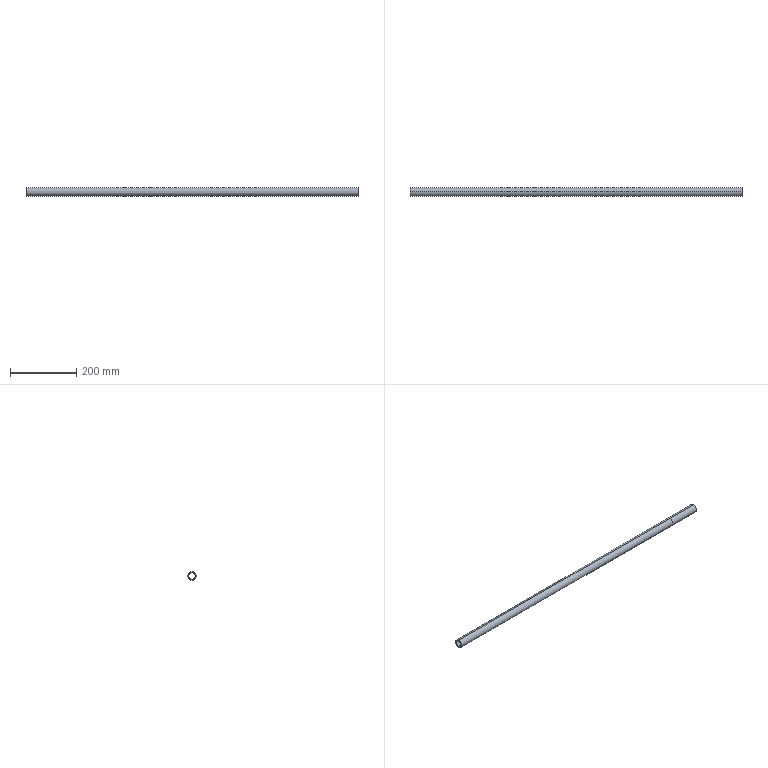Part | STEP file | 51E-01163JG10 | 1 solid | 9 faces | box 1000 x 25.4 x 25.4 mm | volume 190883 mm3 | cylinder 6 | plane 3 | commonest cylinder face diameters 19.8 x2 22.2 x2 25.4 x2
STEP:
#1=CARTESIAN_POINT('',(900.,0.,11.1));
#2=VERTEX_POINT('',#1);
#3=CARTESIAN_POINT('',(900.,0.,-11.1));
#4=VERTEX_POINT('',#3);
#5=CARTESIAN_POINT('',(900.,0.,0.));
#6=DIRECTION('',(1.,0.,0.));
#7=AXIS2_PLACEMENT_3D('',#5,#6,$);
#8=CIRCLE('',#7,11.1);
#9=EDGE_CURVE('',#2,#4,#8,.T.);
#10=ORIENTED_EDGE('',*,*,#9,.F.);
#11=CARTESIAN_POINT('',(1000.,0.,11.1));
#12=VERTEX_POINT('',#11);
#13=CARTESIAN_POINT('',(900.,0.,11.1));
#14=DIRECTION('',(1.,0.,0.));
#15=VECTOR('',#14,1.);
#16=LINE('',#13,#15);
#17=EDGE_CURVE('',#2,#12,#16,.T.);
#18=ORIENTED_EDGE('',*,*,#17,.T.);
#19=CARTESIAN_POINT('',(1000.,0.,-11.1));
#20=VERTEX_POINT('',#19);
#21=CARTESIAN_POINT('',(1000.,0.,0.));
#22=DIRECTION('',(1.,0.,0.));
#23=AXIS2_PLACEMENT_3D('',#21,#22,$);
#24=CIRCLE('',#23,11.1);
#25=EDGE_CURVE('',#12,#20,#24,.T.);
#26=ORIENTED_EDGE('',*,*,#25,.T.);
#27=CARTESIAN_POINT('',(900.,0.,-11.1));
#28=DIRECTION('',(1.,0.,0.));
#29=VECTOR('',#28,1.);
#30=LINE('',#27,#29);
#31=EDGE_CURVE('',#4,#20,#30,.T.);
#32=ORIENTED_EDGE('',*,*,#31,.F.);
#33=EDGE_LOOP('',(#10,#18,#26,#32));
#34=FACE_OUTER_BOUND('',#33,.T.);
#35=CARTESIAN_POINT('',(900.,0.,0.));
#36=DIRECTION('',(1.,0.,0.));
#37=DIRECTION('',(0.,0.,1.));
#38=AXIS2_PLACEMENT_3D('',#35,#36,#37);
#39=CYLINDRICAL_SURFACE('',#38,11.1);
#40=ADVANCED_FACE('',(#34),#39,.F.);
#41=CARTESIAN_POINT('',(900.,0.,0.));
#42=DIRECTION('',(1.,0.,0.));
#43=AXIS2_PLACEMENT_3D('',#41,#42,$);
#44=CIRCLE('',#43,11.1);
#45=EDGE_CURVE('',#4,#2,#44,.T.);
#46=ORIENTED_EDGE('',*,*,#45,.T.);
#47=ORIENTED_EDGE('',*,*,#9,.T.);
#48=EDGE_LOOP('',(#46,#47));
#49=FACE_OUTER_BOUND('',#48,.T.);
#50=CARTESIAN_POINT('',(900.,0.,9.9));
#51=VERTEX_POINT('',#50);
#52=CARTESIAN_POINT('',(900.,0.,-9.9));
#53=VERTEX_POINT('',#52);
#54=CARTESIAN_POINT('',(900.,0.,0.));
#55=DIRECTION('',(1.,0.,0.));
#56=AXIS2_PLACEMENT_3D('',#54,#55,$);
#57=CIRCLE('',#56,9.9);
#58=EDGE_CURVE('',#51,#53,#57,.T.);
#59=ORIENTED_EDGE('',*,*,#58,.F.);
#60=CARTESIAN_POINT('',(900.,0.,0.));
#61=DIRECTION('',(1.,0.,0.));
#62=AXIS2_PLACEMENT_3D('',#60,#61,$);
#63=CIRCLE('',#62,9.9);
#64=EDGE_CURVE('',#53,#51,#63,.T.);
#65=ORIENTED_EDGE('',*,*,#64,.F.);
#66=EDGE_LOOP('',(#59,#65));
#67=FACE_BOUND('',#66,.T.);
#68=CARTESIAN_POINT('',(900.,0.,0.));
#69=DIRECTION('',(1.,0.,0.));
#70=DIRECTION('',(0.,0.,-1.));
#71=AXIS2_PLACEMENT_3D('',#68,#69,#70);
#72=PLANE('',#71);
#73=ADVANCED_FACE('',(#49,#67),#72,.T.);
#74=ORIENTED_EDGE('',*,*,#17,.F.);
#75=ORIENTED_EDGE('',*,*,#45,.F.);
#76=ORIENTED_EDGE('',*,*,#31,.T.);
#77=CARTESIAN_POINT('',(1000.,0.,0.));
#78=DIRECTION('',(1.,0.,0.));
#79=AXIS2_PLACEMENT_3D('',#77,#78,$);
#80=CIRCLE('',#79,11.1);
#81=EDGE_CURVE('',#20,#12,#80,.T.);
#82=ORIENTED_EDGE('',*,*,#81,.T.);
#83=EDGE_LOOP('',(#74,#75,#76,#82));
#84=FACE_OUTER_BOUND('',#83,.T.);
#85=CARTESIAN_POINT('',(900.,0.,0.));
#86=DIRECTION('',(1.,0.,0.));
#87=DIRECTION('',(0.,0.,-1.));
#88=AXIS2_PLACEMENT_3D('',#85,#86,#87);
#89=CYLINDRICAL_SURFACE('',#88,11.1);
#90=ADVANCED_FACE('',(#84),#89,.F.);
#91=CARTESIAN_POINT('',(1000.,0.,12.7));
#92=VERTEX_POINT('',#91);
#93=CARTESIAN_POINT('',(1000.,0.,-12.7));
#94=VERTEX_POINT('',#93);
#95=CARTESIAN_POINT('',(1000.,0.,0.));
#96=DIRECTION('',(1.,0.,0.));
#97=AXIS2_PLACEMENT_3D('',#95,#96,$);
#98=CIRCLE('',#97,12.7);
#99=EDGE_CURVE('',#92,#94,#98,.T.);
#100=ORIENTED_EDGE('',*,*,#99,.T.);
#101=CARTESIAN_POINT('',(1000.,0.,0.));
#102=DIRECTION('',(1.,0.,0.));
#103=AXIS2_PLACEMENT_3D('',#101,#102,$);
#104=CIRCLE('',#103,12.7);
#105=EDGE_CURVE('',#94,#92,#104,.T.);
#106=ORIENTED_EDGE('',*,*,#105,.T.);
#107=EDGE_LOOP('',(#100,#106));
#108=FACE_OUTER_BOUND('',#107,.T.);
#109=ORIENTED_EDGE('',*,*,#81,.F.);
#110=ORIENTED_EDGE('',*,*,#25,.F.);
#111=EDGE_LOOP('',(#109,#110));
#112=FACE_BOUND('',#111,.T.);
#113=CARTESIAN_POINT('',(1000.,0.,0.));
#114=DIRECTION('',(1.,0.,0.));
#115=DIRECTION('',(0.,0.,-1.));
#116=AXIS2_PLACEMENT_3D('',#113,#114,#115);
#117=PLANE('',#116);
#118=ADVANCED_FACE('',(#108,#112),#117,.T.);
#119=ORIENTED_EDGE('',*,*,#58,.T.);
#120=CARTESIAN_POINT('',(0.,0.,-9.9));
#121=VERTEX_POINT('',#120);
#122=CARTESIAN_POINT('',(1000.,0.,-9.9));
#123=DIRECTION('',(-1.,0.,0.));
#124=VECTOR('',#123,1.);
#125=LINE('',#122,#124);
#126=EDGE_CURVE('',#53,#121,#125,.T.);
#127=ORIENTED_EDGE('',*,*,#126,.T.);
#128=CARTESIAN_POINT('',(0.,0.,9.9));
#129=VERTEX_POINT('',#128);
#130=CARTESIAN_POINT('',(0.,0.,0.));
#131=DIRECTION('',(-1.,0.,0.));
#132=AXIS2_PLACEMENT_3D('',#130,#131,$);
#133=CIRCLE('',#132,9.9);
#134=EDGE_CURVE('',#129,#121,#133,.F.);
#135=ORIENTED_EDGE('',*,*,#134,.F.);
#136=CARTESIAN_POINT('',(1000.,0.,9.9));
#137=DIRECTION('',(-1.,0.,0.));
#138=VECTOR('',#137,1.);
#139=LINE('',#136,#138);
#140=EDGE_CURVE('',#51,#129,#139,.T.);
#141=ORIENTED_EDGE('',*,*,#140,.F.);
#142=EDGE_LOOP('',(#119,#127,#135,#141));
#143=FACE_OUTER_BOUND('',#142,.T.);
#144=CARTESIAN_POINT('',(1000.,0.,0.));
#145=DIRECTION('',(-1.,0.,0.));
#146=DIRECTION('',(0.,0.,-1.));
#147=AXIS2_PLACEMENT_3D('',#144,#145,#146);
#148=CYLINDRICAL_SURFACE('',#147,9.9);
#149=ADVANCED_FACE('',(#143),#148,.F.);
#150=ORIENTED_EDGE('',*,*,#126,.F.);
#151=ORIENTED_EDGE('',*,*,#64,.T.);
#152=ORIENTED_EDGE('',*,*,#140,.T.);
#153=CARTESIAN_POINT('',(0.,0.,0.));
#154=DIRECTION('',(-1.,0.,0.));
#155=AXIS2_PLACEMENT_3D('',#153,#154,$);
#156=CIRCLE('',#155,9.9);
#157=EDGE_CURVE('',#121,#129,#156,.F.);
#158=ORIENTED_EDGE('',*,*,#157,.F.);
#159=EDGE_LOOP('',(#150,#151,#152,#158));
#160=FACE_OUTER_BOUND('',#159,.T.);
#161=CARTESIAN_POINT('',(1000.,0.,0.));
#162=DIRECTION('',(-1.,0.,0.));
#163=DIRECTION('',(0.,0.,1.));
#164=AXIS2_PLACEMENT_3D('',#161,#162,#163);
#165=CYLINDRICAL_SURFACE('',#164,9.9);
#166=ADVANCED_FACE('',(#160),#165,.F.);
#167=CARTESIAN_POINT('',(0.,0.,-12.7));
#168=VERTEX_POINT('',#167);
#169=CARTESIAN_POINT('',(1000.,0.,-12.7));
#170=DIRECTION('',(-1.,0.,0.));
#171=VECTOR('',#170,1.);
#172=LINE('',#169,#171);
#173=EDGE_CURVE('',#94,#168,#172,.T.);
#174=ORIENTED_EDGE('',*,*,#173,.F.);
#175=ORIENTED_EDGE('',*,*,#99,.F.);
#176=CARTESIAN_POINT('',(0.,0.,12.7));
#177=VERTEX_POINT('',#176);
#178=CARTESIAN_POINT('',(1000.,0.,12.7));
#179=DIRECTION('',(-1.,0.,0.));
#180=VECTOR('',#179,1.);
#181=LINE('',#178,#180);
#182=EDGE_CURVE('',#92,#177,#181,.T.);
#183=ORIENTED_EDGE('',*,*,#182,.T.);
#184=CARTESIAN_POINT('',(0.,0.,0.));
#185=DIRECTION('',(-1.,0.,0.));
#186=AXIS2_PLACEMENT_3D('',#184,#185,$);
#187=CIRCLE('',#186,12.7);
#188=EDGE_CURVE('',#177,#168,#187,.F.);
#189=ORIENTED_EDGE('',*,*,#188,.T.);
#190=EDGE_LOOP('',(#174,#175,#183,#189));
#191=FACE_OUTER_BOUND('',#190,.T.);
#192=CARTESIAN_POINT('',(1000.,0.,0.));
#193=DIRECTION('',(-1.,0.,0.));
#194=DIRECTION('',(0.,0.,-1.));
#195=AXIS2_PLACEMENT_3D('',#192,#193,#194);
#196=CYLINDRICAL_SURFACE('',#195,12.7);
#197=ADVANCED_FACE('',(#191),#196,.T.);
#198=ORIENTED_EDGE('',*,*,#105,.F.);
#199=ORIENTED_EDGE('',*,*,#173,.T.);
#200=CARTESIAN_POINT('',(0.,0.,0.));
#201=DIRECTION('',(-1.,0.,0.));
#202=AXIS2_PLACEMENT_3D('',#200,#201,$);
#203=CIRCLE('',#202,12.7);
#204=EDGE_CURVE('',#168,#177,#203,.F.);
#205=ORIENTED_EDGE('',*,*,#204,.T.);
#206=ORIENTED_EDGE('',*,*,#182,.F.);
#207=EDGE_LOOP('',(#198,#199,#205,#206));
#208=FACE_OUTER_BOUND('',#207,.T.);
#209=CARTESIAN_POINT('',(1000.,0.,0.));
#210=DIRECTION('',(-1.,0.,0.));
#211=DIRECTION('',(0.,0.,1.));
#212=AXIS2_PLACEMENT_3D('',#209,#210,#211);
#213=CYLINDRICAL_SURFACE('',#212,12.7);
#214=ADVANCED_FACE('',(#208),#213,.T.);
#215=ORIENTED_EDGE('',*,*,#188,.F.);
#216=ORIENTED_EDGE('',*,*,#204,.F.);
#217=EDGE_LOOP('',(#215,#216));
#218=FACE_OUTER_BOUND('',#217,.T.);
#219=ORIENTED_EDGE('',*,*,#134,.T.);
#220=ORIENTED_EDGE('',*,*,#157,.T.);
#221=EDGE_LOOP('',(#219,#220));
#222=FACE_BOUND('',#221,.T.);
#223=CARTESIAN_POINT('',(0.,0.,0.));
#224=DIRECTION('',(1.,0.,0.));
#225=DIRECTION('',(0.,0.,-1.));
#226=AXIS2_PLACEMENT_3D('',#223,#224,#225);
#227=PLANE('',#226);
#228=ADVANCED_FACE('',(#218,#222),#227,.F.);
#229=CLOSED_SHELL('',(#40,#73,#90,#118,#149,#166,#197,#214,#228));
#230=MANIFOLD_SOLID_BREP('',#229);
#231=(LENGTH_UNIT()NAMED_UNIT(*)SI_UNIT(.MILLI.,.METRE.));
#232=UNCERTAINTY_MEASURE_WITH_UNIT(LENGTH_MEASURE(0.005),#231,'','');
#233=(NAMED_UNIT(*)PLANE_ANGLE_UNIT()SI_UNIT($,.RADIAN.));
#234=(NAMED_UNIT(*)SI_UNIT($,.STERADIAN.)SOLID_ANGLE_UNIT());
#235=(GEOMETRIC_REPRESENTATION_CONTEXT(3)GLOBAL_UNCERTAINTY_ASSIGNED_CONTEXT((#232))GLOBAL_UNIT_ASSIGNED_CONTEXT((#231,#233,#234))REPRESENTATION_CONTEXT('',''));
#236=ADVANCED_BREP_SHAPE_REPRESENTATION('',(#230),#235);